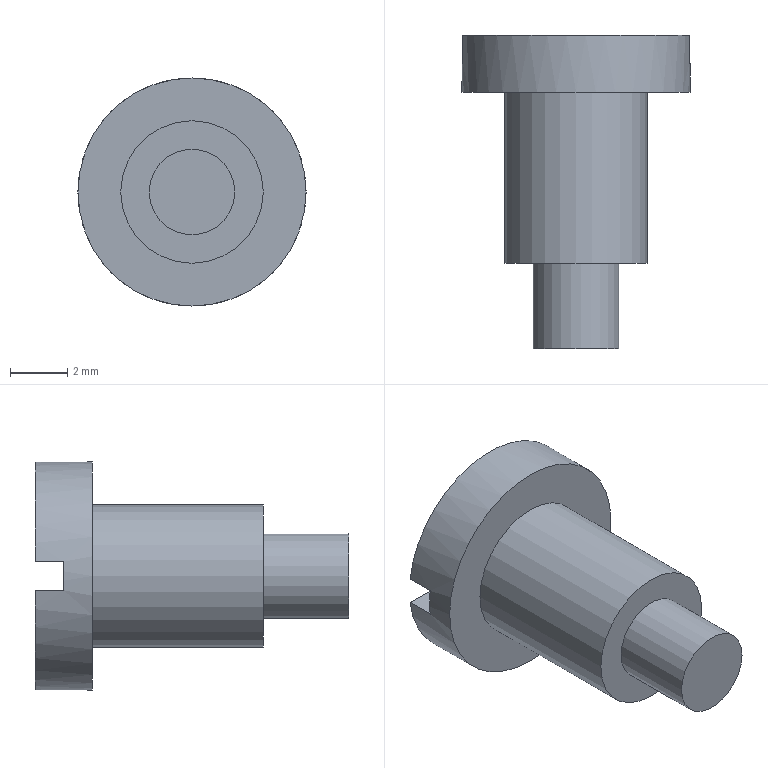Part | STEP file | 2-09.5 | 1 solid | 11 faces | box 8 x 11 x 8 mm | volume 231.567 mm3 | plane 8 | cylinder 3 | commonest cylinder face diameters 3 x1 5 x1 8 x1
STEP:
#1=CARTESIAN_POINT('',(0.,0.,0.));
#2=DIRECTION('',(0.,0.,1.));
#3=DIRECTION('',(1.,0.,0.));
#4=AXIS2_PLACEMENT_3D('',#1,#2,#3);
#5=CARTESIAN_POINT('',(2.5,0.,0.));
#6=VERTEX_POINT('',#5);
#7=CARTESIAN_POINT('',(0.,0.,0.));
#8=DIRECTION('',(0.,-1.,0.));
#9=DIRECTION('',(1.,0.,0.));
#10=AXIS2_PLACEMENT_3D('',#7,#8,#9);
#11=CIRCLE('',#10,2.5);
#12=CARTESIAN_POINT('',(0.,0.,0.));
#13=DIRECTION('',(0.,-1.,0.));
#14=DIRECTION('',(1.,0.,0.));
#15=AXIS2_PLACEMENT_3D('',#12,#13,#14);
#16=CYLINDRICAL_SURFACE('',#15,2.5);
#17=CARTESIAN_POINT('',(0.,0.));
#18=DIRECTION('',(1.,0.));
#19=VECTOR('',#18,1.);
#20=LINE('',#17,#19);
#21=(GEOMETRIC_REPRESENTATION_CONTEXT(2)PARAMETRIC_REPRESENTATION_CONTEXT()REPRESENTATION_CONTEXT('',''));
#22=DEFINITIONAL_REPRESENTATION('',(#20),#21);
#23=PCURVE('',#16,#22);
#24=CARTESIAN_POINT('',(-1.072,0.,0.));
#25=DIRECTION('',(0.,-1.,0.));
#26=DIRECTION('',(1.,0.,0.));
#27=AXIS2_PLACEMENT_3D('',#24,#25,#26);
#28=PLANE('',#27);
#29=CARTESIAN_POINT('',(1.072,0.));
#30=DIRECTION('',(1.,0.));
#31=AXIS2_PLACEMENT_2D('',#29,#30);
#32=CIRCLE('',#31,2.5);
#33=(GEOMETRIC_REPRESENTATION_CONTEXT(2)PARAMETRIC_REPRESENTATION_CONTEXT()REPRESENTATION_CONTEXT('',''));
#34=DEFINITIONAL_REPRESENTATION('',(#32),#33);
#35=PCURVE('',#28,#34);
#36=SURFACE_CURVE('',#11,(#23,#35),.PCURVE_S1.);
#37=EDGE_CURVE('',#6,#6,#36,.T.);
#38=ORIENTED_EDGE('',*,*,#37,.T.);
#39=CARTESIAN_POINT('',(2.5,-6.,0.));
#40=VERTEX_POINT('',#39);
#41=CARTESIAN_POINT('',(2.5,0.,0.));
#42=DIRECTION('',(0.,-1.,0.));
#43=VECTOR('',#42,1.);
#44=LINE('',#41,#43);
#45=CARTESIAN_POINT('',(6.283,0.));
#46=DIRECTION('',(0.,1.));
#47=VECTOR('',#46,1.);
#48=LINE('',#45,#47);
#49=(GEOMETRIC_REPRESENTATION_CONTEXT(2)PARAMETRIC_REPRESENTATION_CONTEXT()REPRESENTATION_CONTEXT('',''));
#50=DEFINITIONAL_REPRESENTATION('',(#48),#49);
#51=PCURVE('',#16,#50);
#52=CARTESIAN_POINT('',(0.,0.));
#53=DIRECTION('',(0.,1.));
#54=VECTOR('',#53,1.);
#55=LINE('',#52,#54);
#56=(GEOMETRIC_REPRESENTATION_CONTEXT(2)PARAMETRIC_REPRESENTATION_CONTEXT()REPRESENTATION_CONTEXT('',''));
#57=DEFINITIONAL_REPRESENTATION('',(#55),#56);
#58=PCURVE('',#16,#57);
#59=SEAM_CURVE('',#44,(#51,#58),.PCURVE_S1.);
#60=EDGE_CURVE('',#6,#40,#59,.T.);
#61=ORIENTED_EDGE('',*,*,#60,.T.);
#62=CARTESIAN_POINT('',(0.,-6.,0.));
#63=DIRECTION('',(0.,-1.,0.));
#64=DIRECTION('',(1.,0.,0.));
#65=AXIS2_PLACEMENT_3D('',#62,#63,#64);
#66=CIRCLE('',#65,2.5);
#67=CARTESIAN_POINT('',(0.,6.));
#68=DIRECTION('',(1.,0.));
#69=VECTOR('',#68,1.);
#70=LINE('',#67,#69);
#71=(GEOMETRIC_REPRESENTATION_CONTEXT(2)PARAMETRIC_REPRESENTATION_CONTEXT()REPRESENTATION_CONTEXT('',''));
#72=DEFINITIONAL_REPRESENTATION('',(#70),#71);
#73=PCURVE('',#16,#72);
#74=CARTESIAN_POINT('',(-0.6699,-6.,0.));
#75=DIRECTION('',(0.,-1.,0.));
#76=DIRECTION('',(1.,0.,0.));
#77=AXIS2_PLACEMENT_3D('',#74,#75,#76);
#78=PLANE('',#77);
#79=CARTESIAN_POINT('',(0.6699,0.));
#80=DIRECTION('',(1.,0.));
#81=AXIS2_PLACEMENT_2D('',#79,#80);
#82=CIRCLE('',#81,2.5);
#83=(GEOMETRIC_REPRESENTATION_CONTEXT(2)PARAMETRIC_REPRESENTATION_CONTEXT()REPRESENTATION_CONTEXT('',''));
#84=DEFINITIONAL_REPRESENTATION('',(#82),#83);
#85=PCURVE('',#78,#84);
#86=SURFACE_CURVE('',#66,(#73,#85),.PCURVE_S1.);
#87=EDGE_CURVE('',#40,#40,#86,.T.);
#88=ORIENTED_EDGE('',*,*,#87,.F.);
#89=ORIENTED_EDGE('',*,*,#60,.F.);
#90=EDGE_LOOP('',(#38,#61,#88,#89));
#91=FACE_BOUND('',#90,.T.);
#92=ADVANCED_FACE('',(#91),#16,.T.);
#93=ORIENTED_EDGE('',*,*,#87,.T.);
#94=EDGE_LOOP('',(#93));
#95=FACE_BOUND('',#94,.T.);
#96=CARTESIAN_POINT('',(1.5,-6.,0.));
#97=VERTEX_POINT('',#96);
#98=CARTESIAN_POINT('',(0.,-6.,0.));
#99=DIRECTION('',(0.,-1.,0.));
#100=DIRECTION('',(1.,0.,0.));
#101=AXIS2_PLACEMENT_3D('',#98,#99,#100);
#102=CIRCLE('',#101,1.5);
#103=CARTESIAN_POINT('',(0.6699,0.));
#104=DIRECTION('',(1.,0.));
#105=AXIS2_PLACEMENT_2D('',#103,#104);
#106=CIRCLE('',#105,1.5);
#107=(GEOMETRIC_REPRESENTATION_CONTEXT(2)PARAMETRIC_REPRESENTATION_CONTEXT()REPRESENTATION_CONTEXT('',''));
#108=DEFINITIONAL_REPRESENTATION('',(#106),#107);
#109=PCURVE('',#78,#108);
#110=CARTESIAN_POINT('',(0.,-6.,0.));
#111=DIRECTION('',(0.,-1.,0.));
#112=DIRECTION('',(1.,0.,0.));
#113=AXIS2_PLACEMENT_3D('',#110,#111,#112);
#114=CYLINDRICAL_SURFACE('',#113,1.5);
#115=CARTESIAN_POINT('',(0.,0.));
#116=DIRECTION('',(1.,0.));
#117=VECTOR('',#116,1.);
#118=LINE('',#115,#117);
#119=(GEOMETRIC_REPRESENTATION_CONTEXT(2)PARAMETRIC_REPRESENTATION_CONTEXT()REPRESENTATION_CONTEXT('',''));
#120=DEFINITIONAL_REPRESENTATION('',(#118),#119);
#121=PCURVE('',#114,#120);
#122=SURFACE_CURVE('',#102,(#109,#121),.PCURVE_S1.);
#123=EDGE_CURVE('',#97,#97,#122,.T.);
#124=ORIENTED_EDGE('',*,*,#123,.F.);
#125=EDGE_LOOP('',(#124));
#126=FACE_BOUND('',#125,.T.);
#127=ADVANCED_FACE('',(#95,#126),#78,.T.);
#128=ORIENTED_EDGE('',*,*,#123,.T.);
#129=CARTESIAN_POINT('',(1.5,-9.,0.));
#130=VERTEX_POINT('',#129);
#131=CARTESIAN_POINT('',(1.5,-6.,0.));
#132=DIRECTION('',(0.,-1.,0.));
#133=VECTOR('',#132,1.);
#134=LINE('',#131,#133);
#135=CARTESIAN_POINT('',(6.283,0.));
#136=DIRECTION('',(0.,1.));
#137=VECTOR('',#136,1.);
#138=LINE('',#135,#137);
#139=(GEOMETRIC_REPRESENTATION_CONTEXT(2)PARAMETRIC_REPRESENTATION_CONTEXT()REPRESENTATION_CONTEXT('',''));
#140=DEFINITIONAL_REPRESENTATION('',(#138),#139);
#141=PCURVE('',#114,#140);
#142=CARTESIAN_POINT('',(0.,0.));
#143=DIRECTION('',(0.,1.));
#144=VECTOR('',#143,1.);
#145=LINE('',#142,#144);
#146=(GEOMETRIC_REPRESENTATION_CONTEXT(2)PARAMETRIC_REPRESENTATION_CONTEXT()REPRESENTATION_CONTEXT('',''));
#147=DEFINITIONAL_REPRESENTATION('',(#145),#146);
#148=PCURVE('',#114,#147);
#149=SEAM_CURVE('',#134,(#141,#148),.PCURVE_S1.);
#150=EDGE_CURVE('',#97,#130,#149,.T.);
#151=ORIENTED_EDGE('',*,*,#150,.T.);
#152=CARTESIAN_POINT('',(0.,-9.,0.));
#153=DIRECTION('',(0.,-1.,0.));
#154=DIRECTION('',(1.,0.,0.));
#155=AXIS2_PLACEMENT_3D('',#152,#153,#154);
#156=CIRCLE('',#155,1.5);
#157=CARTESIAN_POINT('',(0.,3.));
#158=DIRECTION('',(1.,0.));
#159=VECTOR('',#158,1.);
#160=LINE('',#157,#159);
#161=(GEOMETRIC_REPRESENTATION_CONTEXT(2)PARAMETRIC_REPRESENTATION_CONTEXT()REPRESENTATION_CONTEXT('',''));
#162=DEFINITIONAL_REPRESENTATION('',(#160),#161);
#163=PCURVE('',#114,#162);
#164=CARTESIAN_POINT('',(-0.4019,-9.,0.));
#165=DIRECTION('',(0.,-1.,0.));
#166=DIRECTION('',(1.,0.,0.));
#167=AXIS2_PLACEMENT_3D('',#164,#165,#166);
#168=PLANE('',#167);
#169=CARTESIAN_POINT('',(0.4019,0.));
#170=DIRECTION('',(1.,0.));
#171=AXIS2_PLACEMENT_2D('',#169,#170);
#172=CIRCLE('',#171,1.5);
#173=(GEOMETRIC_REPRESENTATION_CONTEXT(2)PARAMETRIC_REPRESENTATION_CONTEXT()REPRESENTATION_CONTEXT('',''));
#174=DEFINITIONAL_REPRESENTATION('',(#172),#173);
#175=PCURVE('',#168,#174);
#176=SURFACE_CURVE('',#156,(#163,#175),.PCURVE_S1.);
#177=EDGE_CURVE('',#130,#130,#176,.T.);
#178=ORIENTED_EDGE('',*,*,#177,.F.);
#179=ORIENTED_EDGE('',*,*,#150,.F.);
#180=EDGE_LOOP('',(#128,#151,#178,#179));
#181=FACE_BOUND('',#180,.T.);
#182=ADVANCED_FACE('',(#181),#114,.T.);
#183=ORIENTED_EDGE('',*,*,#177,.T.);
#184=EDGE_LOOP('',(#183));
#185=FACE_BOUND('',#184,.T.);
#186=ADVANCED_FACE('',(#185),#168,.T.);
#187=CARTESIAN_POINT('',(4.,0.,0.));
#188=VERTEX_POINT('',#187);
#189=CARTESIAN_POINT('',(0.,0.,0.));
#190=DIRECTION('',(0.,-1.,0.));
#191=DIRECTION('',(1.,0.,0.));
#192=AXIS2_PLACEMENT_3D('',#189,#190,#191);
#193=CIRCLE('',#192,4.);
#194=CARTESIAN_POINT('',(1.072,0.));
#195=DIRECTION('',(1.,0.));
#196=AXIS2_PLACEMENT_2D('',#194,#195);
#197=CIRCLE('',#196,4.);
#198=(GEOMETRIC_REPRESENTATION_CONTEXT(2)PARAMETRIC_REPRESENTATION_CONTEXT()REPRESENTATION_CONTEXT('',''));
#199=DEFINITIONAL_REPRESENTATION('',(#197),#198);
#200=PCURVE('',#28,#199);
#201=CARTESIAN_POINT('',(0.,0.,0.));
#202=DIRECTION('',(0.,1.,0.));
#203=DIRECTION('',(1.,0.,0.));
#204=AXIS2_PLACEMENT_3D('',#201,#202,#203);
#205=CYLINDRICAL_SURFACE('',#204,4.);
#206=CARTESIAN_POINT('',(6.283,0.));
#207=DIRECTION('',(-1.,0.));
#208=VECTOR('',#207,1.);
#209=LINE('',#206,#208);
#210=(GEOMETRIC_REPRESENTATION_CONTEXT(2)PARAMETRIC_REPRESENTATION_CONTEXT()REPRESENTATION_CONTEXT('',''));
#211=DEFINITIONAL_REPRESENTATION('',(#209),#210);
#212=PCURVE('',#205,#211);
#213=SURFACE_CURVE('',#193,(#200,#212),.PCURVE_S1.);
#214=EDGE_CURVE('',#188,#188,#213,.T.);
#215=ORIENTED_EDGE('',*,*,#214,.T.);
#216=EDGE_LOOP('',(#215));
#217=FACE_BOUND('',#216,.T.);
#218=ORIENTED_EDGE('',*,*,#37,.F.);
#219=EDGE_LOOP('',(#218));
#220=FACE_BOUND('',#219,.T.);
#221=ADVANCED_FACE('',(#217,#220),#28,.T.);
#222=CARTESIAN_POINT('',(4.,1.,0.));
#223=VERTEX_POINT('',#222);
#224=CARTESIAN_POINT('',(4.,0.,0.));
#225=DIRECTION('',(0.,1.,0.));
#226=VECTOR('',#225,1.);
#227=LINE('',#224,#226);
#228=CARTESIAN_POINT('',(6.283,0.));
#229=DIRECTION('',(0.,1.));
#230=VECTOR('',#229,1.);
#231=LINE('',#228,#230);
#232=(GEOMETRIC_REPRESENTATION_CONTEXT(2)PARAMETRIC_REPRESENTATION_CONTEXT()REPRESENTATION_CONTEXT('',''));
#233=DEFINITIONAL_REPRESENTATION('',(#231),#232);
#234=PCURVE('',#205,#233);
#235=CARTESIAN_POINT('',(0.,0.));
#236=DIRECTION('',(0.,1.));
#237=VECTOR('',#236,1.);
#238=LINE('',#235,#237);
#239=(GEOMETRIC_REPRESENTATION_CONTEXT(2)PARAMETRIC_REPRESENTATION_CONTEXT()REPRESENTATION_CONTEXT('',''));
#240=DEFINITIONAL_REPRESENTATION('',(#238),#239);
#241=PCURVE('',#205,#240);
#242=SEAM_CURVE('',#227,(#234,#241),.PCURVE_S1.);
#243=EDGE_CURVE('',#188,#223,#242,.T.);
#244=ORIENTED_EDGE('',*,*,#243,.T.);
#245=CARTESIAN_POINT('',(3.969,1.,0.5));
#246=VERTEX_POINT('',#245);
#247=CARTESIAN_POINT('',(0.,1.,0.));
#248=DIRECTION('',(0.,1.,0.));
#249=DIRECTION('',(0.9922,0.,0.125));
#250=AXIS2_PLACEMENT_3D('',#247,#248,#249);
#251=CIRCLE('',#250,4.);
#252=CARTESIAN_POINT('',(6.158,1.));
#253=DIRECTION('',(1.,0.));
#254=VECTOR('',#253,1.);
#255=LINE('',#252,#254);
#256=(GEOMETRIC_REPRESENTATION_CONTEXT(2)PARAMETRIC_REPRESENTATION_CONTEXT()REPRESENTATION_CONTEXT('',''));
#257=DEFINITIONAL_REPRESENTATION('',(#255),#256);
#258=PCURVE('',#205,#257);
#259=CARTESIAN_POINT('',(0.,1.,0.));
#260=DIRECTION('',(0.,1.,0.));
#261=DIRECTION('',(0.,0.,-1.));
#262=AXIS2_PLACEMENT_3D('',#259,#260,#261);
#263=PLANE('',#262);
#264=CARTESIAN_POINT('',(0.,0.));
#265=DIRECTION('',(-0.125,-0.9922));
#266=AXIS2_PLACEMENT_2D('',#264,#265);
#267=CIRCLE('',#266,4.);
#268=(GEOMETRIC_REPRESENTATION_CONTEXT(2)PARAMETRIC_REPRESENTATION_CONTEXT()REPRESENTATION_CONTEXT('',''));
#269=DEFINITIONAL_REPRESENTATION('',(#267),#268);
#270=PCURVE('',#263,#269);
#271=SURFACE_CURVE('',#251,(#258,#270),.PCURVE_S1.);
#272=EDGE_CURVE('',#246,#223,#271,.T.);
#273=ORIENTED_EDGE('',*,*,#272,.F.);
#274=CARTESIAN_POINT('',(3.969,2.,0.5));
#275=VERTEX_POINT('',#274);
#276=CARTESIAN_POINT('',(3.969,2.,0.5));
#277=DIRECTION('',(0.,-1.,0.));
#278=VECTOR('',#277,1.);
#279=LINE('',#276,#278);
#280=CARTESIAN_POINT('',(6.158,2.));
#281=DIRECTION('',(0.,-1.));
#282=VECTOR('',#281,1.);
#283=LINE('',#280,#282);
#284=(GEOMETRIC_REPRESENTATION_CONTEXT(2)PARAMETRIC_REPRESENTATION_CONTEXT()REPRESENTATION_CONTEXT('',''));
#285=DEFINITIONAL_REPRESENTATION('',(#283),#284);
#286=PCURVE('',#205,#285);
#287=CARTESIAN_POINT('',(0.,2.,0.5));
#288=DIRECTION('',(0.,0.,-1.));
#289=DIRECTION('',(0.,-1.,0.));
#290=AXIS2_PLACEMENT_3D('',#287,#288,#289);
#291=PLANE('',#290);
#292=CARTESIAN_POINT('',(0.,-3.969));
#293=DIRECTION('',(1.,0.));
#294=VECTOR('',#293,1.);
#295=LINE('',#292,#294);
#296=(GEOMETRIC_REPRESENTATION_CONTEXT(2)PARAMETRIC_REPRESENTATION_CONTEXT()REPRESENTATION_CONTEXT('',''));
#297=DEFINITIONAL_REPRESENTATION('',(#295),#296);
#298=PCURVE('',#291,#297);
#299=SURFACE_CURVE('',#279,(#286,#298),.PCURVE_S1.);
#300=EDGE_CURVE('',#275,#246,#299,.T.);
#301=ORIENTED_EDGE('',*,*,#300,.F.);
#302=CARTESIAN_POINT('',(-3.969,2.,0.5));
#303=VERTEX_POINT('',#302);
#304=CARTESIAN_POINT('',(0.,2.,0.));
#305=DIRECTION('',(0.,-1.,0.));
#306=DIRECTION('',(0.9922,0.,0.125));
#307=AXIS2_PLACEMENT_3D('',#304,#305,#306);
#308=CIRCLE('',#307,4.);
#309=CARTESIAN_POINT('',(6.158,2.));
#310=DIRECTION('',(-1.,0.));
#311=VECTOR('',#310,1.);
#312=LINE('',#309,#311);
#313=(GEOMETRIC_REPRESENTATION_CONTEXT(2)PARAMETRIC_REPRESENTATION_CONTEXT()REPRESENTATION_CONTEXT('',''));
#314=DEFINITIONAL_REPRESENTATION('',(#312),#313);
#315=PCURVE('',#205,#314);
#316=CARTESIAN_POINT('',(0.,2.,0.));
#317=DIRECTION('',(0.,-1.,0.));
#318=DIRECTION('',(1.,0.,0.));
#319=AXIS2_PLACEMENT_3D('',#316,#317,#318);
#320=PLANE('',#319);
#321=CARTESIAN_POINT('',(0.,0.));
#322=DIRECTION('',(0.9922,0.125));
#323=AXIS2_PLACEMENT_2D('',#321,#322);
#324=CIRCLE('',#323,4.);
#325=(GEOMETRIC_REPRESENTATION_CONTEXT(2)PARAMETRIC_REPRESENTATION_CONTEXT()REPRESENTATION_CONTEXT('',''));
#326=DEFINITIONAL_REPRESENTATION('',(#324),#325);
#327=PCURVE('',#320,#326);
#328=SURFACE_CURVE('',#308,(#315,#327),.PCURVE_S1.);
#329=EDGE_CURVE('',#275,#303,#328,.T.);
#330=ORIENTED_EDGE('',*,*,#329,.T.);
#331=CARTESIAN_POINT('',(-3.969,1.,0.5));
#332=VERTEX_POINT('',#331);
#333=CARTESIAN_POINT('',(-3.969,1.,0.5));
#334=DIRECTION('',(0.,1.,0.));
#335=VECTOR('',#334,1.);
#336=LINE('',#333,#335);
#337=CARTESIAN_POINT('',(3.267,1.));
#338=DIRECTION('',(0.,1.));
#339=VECTOR('',#338,1.);
#340=LINE('',#337,#339);
#341=(GEOMETRIC_REPRESENTATION_CONTEXT(2)PARAMETRIC_REPRESENTATION_CONTEXT()REPRESENTATION_CONTEXT('',''));
#342=DEFINITIONAL_REPRESENTATION('',(#340),#341);
#343=PCURVE('',#205,#342);
#344=CARTESIAN_POINT('',(1.,3.969));
#345=DIRECTION('',(-1.,0.));
#346=VECTOR('',#345,1.);
#347=LINE('',#344,#346);
#348=(GEOMETRIC_REPRESENTATION_CONTEXT(2)PARAMETRIC_REPRESENTATION_CONTEXT()REPRESENTATION_CONTEXT('',''));
#349=DEFINITIONAL_REPRESENTATION('',(#347),#348);
#350=PCURVE('',#291,#349);
#351=SURFACE_CURVE('',#336,(#343,#350),.PCURVE_S1.);
#352=EDGE_CURVE('',#332,#303,#351,.T.);
#353=ORIENTED_EDGE('',*,*,#352,.F.);
#354=CARTESIAN_POINT('',(-3.969,1.,-0.5));
#355=VERTEX_POINT('',#354);
#356=CARTESIAN_POINT('',(0.,1.,0.));
#357=DIRECTION('',(0.,1.,0.));
#358=DIRECTION('',(-0.9922,0.,-0.125));
#359=AXIS2_PLACEMENT_3D('',#356,#357,#358);
#360=CIRCLE('',#359,4.);
#361=CARTESIAN_POINT('',(3.016,1.));
#362=DIRECTION('',(1.,0.));
#363=VECTOR('',#362,1.);
#364=LINE('',#361,#363);
#365=(GEOMETRIC_REPRESENTATION_CONTEXT(2)PARAMETRIC_REPRESENTATION_CONTEXT()REPRESENTATION_CONTEXT('',''));
#366=DEFINITIONAL_REPRESENTATION('',(#364),#365);
#367=PCURVE('',#205,#366);
#368=CARTESIAN_POINT('',(0.,0.));
#369=DIRECTION('',(0.125,0.9922));
#370=AXIS2_PLACEMENT_2D('',#368,#369);
#371=CIRCLE('',#370,4.);
#372=(GEOMETRIC_REPRESENTATION_CONTEXT(2)PARAMETRIC_REPRESENTATION_CONTEXT()REPRESENTATION_CONTEXT('',''));
#373=DEFINITIONAL_REPRESENTATION('',(#371),#372);
#374=PCURVE('',#263,#373);
#375=SURFACE_CURVE('',#360,(#367,#374),.PCURVE_S1.);
#376=EDGE_CURVE('',#355,#332,#375,.T.);
#377=ORIENTED_EDGE('',*,*,#376,.F.);
#378=CARTESIAN_POINT('',(-3.969,2.,-0.5));
#379=VERTEX_POINT('',#378);
#380=CARTESIAN_POINT('',(-3.969,2.,-0.5));
#381=DIRECTION('',(0.,-1.,0.));
#382=VECTOR('',#381,1.);
#383=LINE('',#380,#382);
#384=CARTESIAN_POINT('',(3.016,2.));
#385=DIRECTION('',(0.,-1.));
#386=VECTOR('',#385,1.);
#387=LINE('',#384,#386);
#388=(GEOMETRIC_REPRESENTATION_CONTEXT(2)PARAMETRIC_REPRESENTATION_CONTEXT()REPRESENTATION_CONTEXT('',''));
#389=DEFINITIONAL_REPRESENTATION('',(#387),#388);
#390=PCURVE('',#205,#389);
#391=CARTESIAN_POINT('',(0.,2.,-0.5));
#392=DIRECTION('',(0.,0.,1.));
#393=DIRECTION('',(0.,1.,0.));
#394=AXIS2_PLACEMENT_3D('',#391,#392,#393);
#395=PLANE('',#394);
#396=CARTESIAN_POINT('',(0.,3.969));
#397=DIRECTION('',(-1.,0.));
#398=VECTOR('',#397,1.);
#399=LINE('',#396,#398);
#400=(GEOMETRIC_REPRESENTATION_CONTEXT(2)PARAMETRIC_REPRESENTATION_CONTEXT()REPRESENTATION_CONTEXT('',''));
#401=DEFINITIONAL_REPRESENTATION('',(#399),#400);
#402=PCURVE('',#395,#401);
#403=SURFACE_CURVE('',#383,(#390,#402),.PCURVE_S1.);
#404=EDGE_CURVE('',#379,#355,#403,.T.);
#405=ORIENTED_EDGE('',*,*,#404,.F.);
#406=CARTESIAN_POINT('',(3.969,2.,-0.5));
#407=VERTEX_POINT('',#406);
#408=CARTESIAN_POINT('',(0.,2.,0.));
#409=DIRECTION('',(0.,-1.,0.));
#410=DIRECTION('',(-0.9922,0.,-0.125));
#411=AXIS2_PLACEMENT_3D('',#408,#409,#410);
#412=CIRCLE('',#411,4.);
#413=CARTESIAN_POINT('',(3.016,2.));
#414=DIRECTION('',(-1.,0.));
#415=VECTOR('',#414,1.);
#416=LINE('',#413,#415);
#417=(GEOMETRIC_REPRESENTATION_CONTEXT(2)PARAMETRIC_REPRESENTATION_CONTEXT()REPRESENTATION_CONTEXT('',''));
#418=DEFINITIONAL_REPRESENTATION('',(#416),#417);
#419=PCURVE('',#205,#418);
#420=CARTESIAN_POINT('',(0.,2.,0.));
#421=DIRECTION('',(0.,-1.,0.));
#422=DIRECTION('',(1.,0.,0.));
#423=AXIS2_PLACEMENT_3D('',#420,#421,#422);
#424=PLANE('',#423);
#425=CARTESIAN_POINT('',(0.,0.));
#426=DIRECTION('',(-0.9922,-0.125));
#427=AXIS2_PLACEMENT_2D('',#425,#426);
#428=CIRCLE('',#427,4.);
#429=(GEOMETRIC_REPRESENTATION_CONTEXT(2)PARAMETRIC_REPRESENTATION_CONTEXT()REPRESENTATION_CONTEXT('',''));
#430=DEFINITIONAL_REPRESENTATION('',(#428),#429);
#431=PCURVE('',#424,#430);
#432=SURFACE_CURVE('',#412,(#419,#431),.PCURVE_S1.);
#433=EDGE_CURVE('',#379,#407,#432,.T.);
#434=ORIENTED_EDGE('',*,*,#433,.T.);
#435=CARTESIAN_POINT('',(3.969,1.,-0.5));
#436=VERTEX_POINT('',#435);
#437=CARTESIAN_POINT('',(3.969,1.,-0.5));
#438=DIRECTION('',(0.,1.,0.));
#439=VECTOR('',#438,1.);
#440=LINE('',#437,#439);
#441=CARTESIAN_POINT('',(0.1253,1.));
#442=DIRECTION('',(0.,1.));
#443=VECTOR('',#442,1.);
#444=LINE('',#441,#443);
#445=(GEOMETRIC_REPRESENTATION_CONTEXT(2)PARAMETRIC_REPRESENTATION_CONTEXT()REPRESENTATION_CONTEXT('',''));
#446=DEFINITIONAL_REPRESENTATION('',(#444),#445);
#447=PCURVE('',#205,#446);
#448=CARTESIAN_POINT('',(-1.,-3.969));
#449=DIRECTION('',(1.,0.));
#450=VECTOR('',#449,1.);
#451=LINE('',#448,#450);
#452=(GEOMETRIC_REPRESENTATION_CONTEXT(2)PARAMETRIC_REPRESENTATION_CONTEXT()REPRESENTATION_CONTEXT('',''));
#453=DEFINITIONAL_REPRESENTATION('',(#451),#452);
#454=PCURVE('',#395,#453);
#455=SURFACE_CURVE('',#440,(#447,#454),.PCURVE_S1.);
#456=EDGE_CURVE('',#436,#407,#455,.T.);
#457=ORIENTED_EDGE('',*,*,#456,.F.);
#458=CARTESIAN_POINT('',(0.,1.,0.));
#459=DIRECTION('',(0.,1.,0.));
#460=DIRECTION('',(1.,0.,0.));
#461=AXIS2_PLACEMENT_3D('',#458,#459,#460);
#462=CIRCLE('',#461,4.);
#463=CARTESIAN_POINT('',(0.,1.));
#464=DIRECTION('',(1.,0.));
#465=VECTOR('',#464,1.);
#466=LINE('',#463,#465);
#467=(GEOMETRIC_REPRESENTATION_CONTEXT(2)PARAMETRIC_REPRESENTATION_CONTEXT()REPRESENTATION_CONTEXT('',''));
#468=DEFINITIONAL_REPRESENTATION('',(#466),#467);
#469=PCURVE('',#205,#468);
#470=CARTESIAN_POINT('',(0.,0.));
#471=DIRECTION('',(0.,-1.));
#472=AXIS2_PLACEMENT_2D('',#470,#471);
#473=CIRCLE('',#472,4.);
#474=(GEOMETRIC_REPRESENTATION_CONTEXT(2)PARAMETRIC_REPRESENTATION_CONTEXT()REPRESENTATION_CONTEXT('',''));
#475=DEFINITIONAL_REPRESENTATION('',(#473),#474);
#476=PCURVE('',#263,#475);
#477=SURFACE_CURVE('',#462,(#469,#476),.PCURVE_S1.);
#478=EDGE_CURVE('',#223,#436,#477,.T.);
#479=ORIENTED_EDGE('',*,*,#478,.F.);
#480=ORIENTED_EDGE('',*,*,#243,.F.);
#481=ORIENTED_EDGE('',*,*,#214,.F.);
#482=EDGE_LOOP('',(#244,#273,#301,#330,#353,#377,#405,#434,#457,#479,#480,#481));
#483=FACE_BOUND('',#482,.T.);
#484=ADVANCED_FACE('',(#483),#205,.T.);
#485=ORIENTED_EDGE('',*,*,#433,.T.);
#486=CARTESIAN_POINT('',(3.969,2.,-0.5));
#487=DIRECTION('',(-1.,0.,0.));
#488=VECTOR('',#487,1.);
#489=LINE('',#486,#488);
#490=CARTESIAN_POINT('',(3.969,-0.5));
#491=DIRECTION('',(-1.,0.));
#492=VECTOR('',#491,1.);
#493=LINE('',#490,#492);
#494=(GEOMETRIC_REPRESENTATION_CONTEXT(2)PARAMETRIC_REPRESENTATION_CONTEXT()REPRESENTATION_CONTEXT('',''));
#495=DEFINITIONAL_REPRESENTATION('',(#493),#494);
#496=PCURVE('',#424,#495);
#497=CARTESIAN_POINT('',(0.,-3.969));
#498=DIRECTION('',(0.,1.));
#499=VECTOR('',#498,1.);
#500=LINE('',#497,#499);
#501=(GEOMETRIC_REPRESENTATION_CONTEXT(2)PARAMETRIC_REPRESENTATION_CONTEXT()REPRESENTATION_CONTEXT('',''));
#502=DEFINITIONAL_REPRESENTATION('',(#500),#501);
#503=PCURVE('',#395,#502);
#504=SURFACE_CURVE('',#489,(#496,#503),.PCURVE_S1.);
#505=EDGE_CURVE('',#407,#379,#504,.T.);
#506=ORIENTED_EDGE('',*,*,#505,.T.);
#507=EDGE_LOOP('',(#485,#506));
#508=FACE_BOUND('',#507,.F.);
#509=ADVANCED_FACE('',(#508),#424,.F.);
#510=ORIENTED_EDGE('',*,*,#329,.T.);
#511=CARTESIAN_POINT('',(-3.969,2.,0.5));
#512=DIRECTION('',(1.,0.,0.));
#513=VECTOR('',#512,1.);
#514=LINE('',#511,#513);
#515=CARTESIAN_POINT('',(-3.969,0.5));
#516=DIRECTION('',(1.,0.));
#517=VECTOR('',#516,1.);
#518=LINE('',#515,#517);
#519=(GEOMETRIC_REPRESENTATION_CONTEXT(2)PARAMETRIC_REPRESENTATION_CONTEXT()REPRESENTATION_CONTEXT('',''));
#520=DEFINITIONAL_REPRESENTATION('',(#518),#519);
#521=PCURVE('',#320,#520);
#522=CARTESIAN_POINT('',(0.,3.969));
#523=DIRECTION('',(0.,-1.));
#524=VECTOR('',#523,1.);
#525=LINE('',#522,#524);
#526=(GEOMETRIC_REPRESENTATION_CONTEXT(2)PARAMETRIC_REPRESENTATION_CONTEXT()REPRESENTATION_CONTEXT('',''));
#527=DEFINITIONAL_REPRESENTATION('',(#525),#526);
#528=PCURVE('',#291,#527);
#529=SURFACE_CURVE('',#514,(#521,#528),.PCURVE_S1.);
#530=EDGE_CURVE('',#303,#275,#529,.T.);
#531=ORIENTED_EDGE('',*,*,#530,.T.);
#532=EDGE_LOOP('',(#510,#531));
#533=FACE_BOUND('',#532,.F.);
#534=ADVANCED_FACE('',(#533),#320,.F.);
#535=CARTESIAN_POINT('',(3.969,1.,0.5));
#536=DIRECTION('',(-1.,0.,0.));
#537=VECTOR('',#536,1.);
#538=LINE('',#535,#537);
#539=CARTESIAN_POINT('',(-0.5,-3.969));
#540=DIRECTION('',(0.,1.));
#541=VECTOR('',#540,1.);
#542=LINE('',#539,#541);
#543=(GEOMETRIC_REPRESENTATION_CONTEXT(2)PARAMETRIC_REPRESENTATION_CONTEXT()REPRESENTATION_CONTEXT('',''));
#544=DEFINITIONAL_REPRESENTATION('',(#542),#543);
#545=PCURVE('',#263,#544);
#546=CARTESIAN_POINT('',(1.,-3.969));
#547=DIRECTION('',(0.,1.));
#548=VECTOR('',#547,1.);
#549=LINE('',#546,#548);
#550=(GEOMETRIC_REPRESENTATION_CONTEXT(2)PARAMETRIC_REPRESENTATION_CONTEXT()REPRESENTATION_CONTEXT('',''));
#551=DEFINITIONAL_REPRESENTATION('',(#549),#550);
#552=PCURVE('',#291,#551);
#553=SURFACE_CURVE('',#538,(#545,#552),.PCURVE_S1.);
#554=EDGE_CURVE('',#246,#332,#553,.T.);
#555=ORIENTED_EDGE('',*,*,#554,.F.);
#556=ORIENTED_EDGE('',*,*,#272,.T.);
#557=ORIENTED_EDGE('',*,*,#478,.T.);
#558=CARTESIAN_POINT('',(3.969,1.,-0.5));
#559=DIRECTION('',(-1.,0.,0.));
#560=VECTOR('',#559,1.);
#561=LINE('',#558,#560);
#562=CARTESIAN_POINT('',(0.5,-3.969));
#563=DIRECTION('',(0.,1.));
#564=VECTOR('',#563,1.);
#565=LINE('',#562,#564);
#566=(GEOMETRIC_REPRESENTATION_CONTEXT(2)PARAMETRIC_REPRESENTATION_CONTEXT()REPRESENTATION_CONTEXT('',''));
#567=DEFINITIONAL_REPRESENTATION('',(#565),#566);
#568=PCURVE('',#263,#567);
#569=CARTESIAN_POINT('',(-1.,-3.969));
#570=DIRECTION('',(0.,1.));
#571=VECTOR('',#570,1.);
#572=LINE('',#569,#571);
#573=(GEOMETRIC_REPRESENTATION_CONTEXT(2)PARAMETRIC_REPRESENTATION_CONTEXT()REPRESENTATION_CONTEXT('',''));
#574=DEFINITIONAL_REPRESENTATION('',(#572),#573);
#575=PCURVE('',#395,#574);
#576=SURFACE_CURVE('',#561,(#568,#575),.PCURVE_S1.);
#577=EDGE_CURVE('',#436,#355,#576,.T.);
#578=ORIENTED_EDGE('',*,*,#577,.T.);
#579=ORIENTED_EDGE('',*,*,#376,.T.);
#580=EDGE_LOOP('',(#555,#556,#557,#578,#579));
#581=FACE_BOUND('',#580,.T.);
#582=ADVANCED_FACE('',(#581),#263,.T.);
#583=ORIENTED_EDGE('',*,*,#577,.F.);
#584=ORIENTED_EDGE('',*,*,#456,.T.);
#585=ORIENTED_EDGE('',*,*,#505,.T.);
#586=ORIENTED_EDGE('',*,*,#404,.T.);
#587=EDGE_LOOP('',(#583,#584,#585,#586));
#588=FACE_BOUND('',#587,.T.);
#589=ADVANCED_FACE('',(#588),#395,.T.);
#590=ORIENTED_EDGE('',*,*,#554,.T.);
#591=ORIENTED_EDGE('',*,*,#352,.T.);
#592=ORIENTED_EDGE('',*,*,#530,.T.);
#593=ORIENTED_EDGE('',*,*,#300,.T.);
#594=EDGE_LOOP('',(#590,#591,#592,#593));
#595=FACE_BOUND('',#594,.T.);
#596=ADVANCED_FACE('',(#595),#291,.T.);
#597=CLOSED_SHELL('',(#92,#127,#182,#186,#221,#484,#509,#534,#582,#589,#596));
#598=MANIFOLD_SOLID_BREP('',#597);
#599=(LENGTH_UNIT()NAMED_UNIT(*)SI_UNIT(.MILLI.,.METRE.));
#600=UNCERTAINTY_MEASURE_WITH_UNIT(LENGTH_MEASURE(0.0000001),#599,'','');
#601=(NAMED_UNIT(*)PLANE_ANGLE_UNIT()SI_UNIT($,.RADIAN.));
#602=(NAMED_UNIT(*)SI_UNIT($,.STERADIAN.)SOLID_ANGLE_UNIT());
#603=(GEOMETRIC_REPRESENTATION_CONTEXT(3)GLOBAL_UNCERTAINTY_ASSIGNED_CONTEXT((#600))GLOBAL_UNIT_ASSIGNED_CONTEXT((#599,#601,#602))REPRESENTATION_CONTEXT('',''));
#604=ADVANCED_BREP_SHAPE_REPRESENTATION('',(#4,#598),#603);